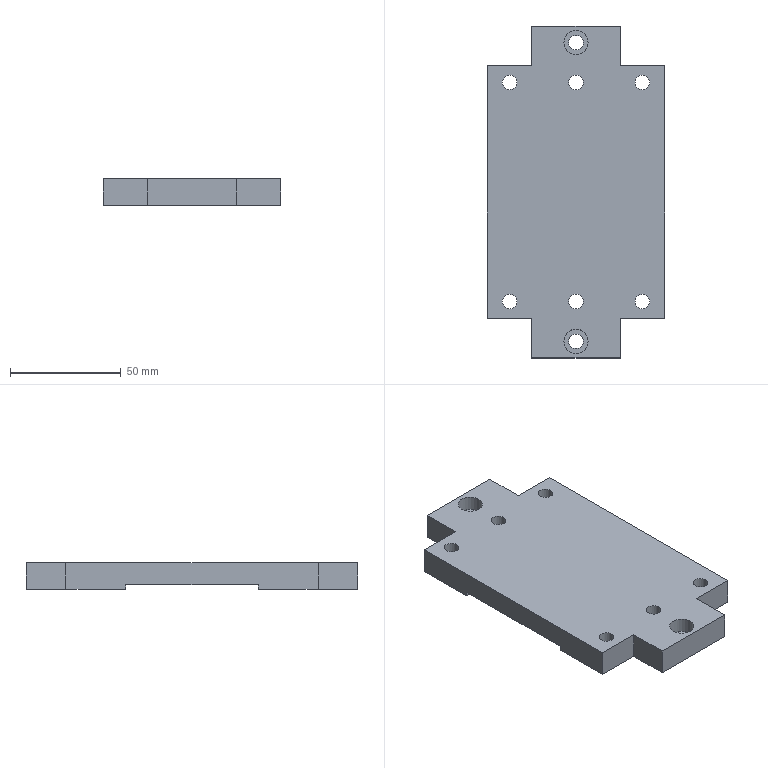Part | NX | 1 solid | 42 faces | box 80 x 150 x 12 mm | volume 110527 mm3 | plane 26 | cylinder 16 | commonest cylinder face diameters 6.6 x8 11 x8
STEP:
#1=CARTESIAN_POINT('',(5.5,67.5,6.));
#2=VERTEX_POINT('',#1);
#3=CARTESIAN_POINT('',(0.,67.5,6.));
#4=DIRECTION('',(0.,0.,1.));
#5=DIRECTION('',(1.,0.,0.));
#6=AXIS2_PLACEMENT_3D('',#3,#4,#5);
#7=CIRCLE('',#6,5.5);
#8=EDGE_CURVE('',#2,#2,#7,.T.);
#9=ORIENTED_EDGE('',*,*,#8,.F.);
#10=EDGE_LOOP('',(#9));
#11=FACE_BOUND('',#10,.T.);
#12=CARTESIAN_POINT('',(5.5,-67.5,6.));
#13=VERTEX_POINT('',#12);
#14=CARTESIAN_POINT('',(0.,-67.5,6.));
#15=DIRECTION('',(0.,0.,1.));
#16=DIRECTION('',(1.,0.,0.));
#17=AXIS2_PLACEMENT_3D('',#14,#15,#16);
#18=CIRCLE('',#17,5.5);
#19=EDGE_CURVE('',#13,#13,#18,.T.);
#20=ORIENTED_EDGE('',*,*,#19,.F.);
#21=EDGE_LOOP('',(#20));
#22=FACE_BOUND('',#21,.T.);
#23=CARTESIAN_POINT('',(-33.3,-49.5,6.));
#24=VERTEX_POINT('',#23);
#25=CARTESIAN_POINT('',(-30.,-49.5,6.));
#26=DIRECTION('',(0.,0.,-1.));
#27=DIRECTION('',(-1.,0.,0.));
#28=AXIS2_PLACEMENT_3D('',#25,#26,#27);
#29=CIRCLE('',#28,3.3);
#30=EDGE_CURVE('',#24,#24,#29,.T.);
#31=ORIENTED_EDGE('',*,*,#30,.T.);
#32=EDGE_LOOP('',(#31));
#33=FACE_BOUND('',#32,.T.);
#34=CARTESIAN_POINT('',(-3.3,-49.5,6.));
#35=VERTEX_POINT('',#34);
#36=CARTESIAN_POINT('',(0.,-49.5,6.));
#37=DIRECTION('',(0.,0.,-1.));
#38=DIRECTION('',(-1.,0.,0.));
#39=AXIS2_PLACEMENT_3D('',#36,#37,#38);
#40=CIRCLE('',#39,3.3);
#41=EDGE_CURVE('',#35,#35,#40,.T.);
#42=ORIENTED_EDGE('',*,*,#41,.T.);
#43=EDGE_LOOP('',(#42));
#44=FACE_BOUND('',#43,.T.);
#45=CARTESIAN_POINT('',(26.7,-49.5,6.));
#46=VERTEX_POINT('',#45);
#47=CARTESIAN_POINT('',(30.,-49.5,6.));
#48=DIRECTION('',(0.,0.,-1.));
#49=DIRECTION('',(-1.,0.,0.));
#50=AXIS2_PLACEMENT_3D('',#47,#48,#49);
#51=CIRCLE('',#50,3.3);
#52=EDGE_CURVE('',#46,#46,#51,.T.);
#53=ORIENTED_EDGE('',*,*,#52,.T.);
#54=EDGE_LOOP('',(#53));
#55=FACE_BOUND('',#54,.T.);
#56=CARTESIAN_POINT('',(-33.3,49.5,6.));
#57=VERTEX_POINT('',#56);
#58=CARTESIAN_POINT('',(-30.,49.5,6.));
#59=DIRECTION('',(0.,0.,-1.));
#60=DIRECTION('',(-1.,0.,0.));
#61=AXIS2_PLACEMENT_3D('',#58,#59,#60);
#62=CIRCLE('',#61,3.3);
#63=EDGE_CURVE('',#57,#57,#62,.T.);
#64=ORIENTED_EDGE('',*,*,#63,.T.);
#65=EDGE_LOOP('',(#64));
#66=FACE_BOUND('',#65,.T.);
#67=CARTESIAN_POINT('',(-3.3,49.5,6.));
#68=VERTEX_POINT('',#67);
#69=CARTESIAN_POINT('',(0.,49.5,6.));
#70=DIRECTION('',(0.,0.,-1.));
#71=DIRECTION('',(-1.,0.,0.));
#72=AXIS2_PLACEMENT_3D('',#69,#70,#71);
#73=CIRCLE('',#72,3.3);
#74=EDGE_CURVE('',#68,#68,#73,.T.);
#75=ORIENTED_EDGE('',*,*,#74,.T.);
#76=EDGE_LOOP('',(#75));
#77=FACE_BOUND('',#76,.T.);
#78=CARTESIAN_POINT('',(26.7,49.5,6.));
#79=VERTEX_POINT('',#78);
#80=CARTESIAN_POINT('',(30.,49.5,6.));
#81=DIRECTION('',(0.,0.,-1.));
#82=DIRECTION('',(-1.,0.,0.));
#83=AXIS2_PLACEMENT_3D('',#80,#81,#82);
#84=CIRCLE('',#83,3.3);
#85=EDGE_CURVE('',#79,#79,#84,.T.);
#86=ORIENTED_EDGE('',*,*,#85,.T.);
#87=EDGE_LOOP('',(#86));
#88=FACE_BOUND('',#87,.T.);
#89=CARTESIAN_POINT('',(-40.,57.,6.));
#90=VERTEX_POINT('',#89);
#91=CARTESIAN_POINT('',(-40.,-57.,6.));
#92=VERTEX_POINT('',#91);
#93=CARTESIAN_POINT('',(-40.,75.,6.));
#94=DIRECTION('',(0.,-1.,0.));
#95=VECTOR('',#94,1000.);
#96=LINE('',#93,#95);
#97=EDGE_CURVE('',#90,#92,#96,.T.);
#98=ORIENTED_EDGE('',*,*,#97,.T.);
#99=CARTESIAN_POINT('',(-20.,-57.,6.));
#100=VERTEX_POINT('',#99);
#101=CARTESIAN_POINT('',(-40.,-57.,6.));
#102=DIRECTION('',(1.,0.,0.));
#103=VECTOR('',#102,1000.);
#104=LINE('',#101,#103);
#105=EDGE_CURVE('',#92,#100,#104,.T.);
#106=ORIENTED_EDGE('',*,*,#105,.T.);
#107=CARTESIAN_POINT('',(-20.,-75.,6.));
#108=VERTEX_POINT('',#107);
#109=CARTESIAN_POINT('',(-20.,-75.,6.));
#110=DIRECTION('',(0.,-1.,0.));
#111=VECTOR('',#110,1000.);
#112=LINE('',#109,#111);
#113=EDGE_CURVE('',#100,#108,#112,.T.);
#114=ORIENTED_EDGE('',*,*,#113,.T.);
#115=CARTESIAN_POINT('',(20.,-75.,6.));
#116=VERTEX_POINT('',#115);
#117=CARTESIAN_POINT('',(-40.,-75.,6.));
#118=DIRECTION('',(1.,0.,0.));
#119=VECTOR('',#118,1000.);
#120=LINE('',#117,#119);
#121=EDGE_CURVE('',#108,#116,#120,.T.);
#122=ORIENTED_EDGE('',*,*,#121,.T.);
#123=CARTESIAN_POINT('',(20.,-57.,6.));
#124=VERTEX_POINT('',#123);
#125=CARTESIAN_POINT('',(20.,-75.,6.));
#126=DIRECTION('',(0.,-1.,0.));
#127=VECTOR('',#126,1000.);
#128=LINE('',#125,#127);
#129=EDGE_CURVE('',#124,#116,#128,.T.);
#130=ORIENTED_EDGE('',*,*,#129,.F.);
#131=CARTESIAN_POINT('',(40.,-57.,6.));
#132=VERTEX_POINT('',#131);
#133=CARTESIAN_POINT('',(40.,-57.,6.));
#134=DIRECTION('',(-1.,0.,0.));
#135=VECTOR('',#134,1000.);
#136=LINE('',#133,#135);
#137=EDGE_CURVE('',#132,#124,#136,.T.);
#138=ORIENTED_EDGE('',*,*,#137,.F.);
#139=CARTESIAN_POINT('',(40.,57.,6.));
#140=VERTEX_POINT('',#139);
#141=CARTESIAN_POINT('',(40.,75.,6.));
#142=DIRECTION('',(0.,1.,0.));
#143=VECTOR('',#142,1000.);
#144=LINE('',#141,#143);
#145=EDGE_CURVE('',#132,#140,#144,.T.);
#146=ORIENTED_EDGE('',*,*,#145,.T.);
#147=CARTESIAN_POINT('',(20.,57.,6.));
#148=VERTEX_POINT('',#147);
#149=CARTESIAN_POINT('',(40.,57.,6.));
#150=DIRECTION('',(-1.,0.,0.));
#151=VECTOR('',#150,1000.);
#152=LINE('',#149,#151);
#153=EDGE_CURVE('',#140,#148,#152,.T.);
#154=ORIENTED_EDGE('',*,*,#153,.T.);
#155=CARTESIAN_POINT('',(20.,75.,6.));
#156=VERTEX_POINT('',#155);
#157=CARTESIAN_POINT('',(20.,75.,6.));
#158=DIRECTION('',(0.,1.,0.));
#159=VECTOR('',#158,1000.);
#160=LINE('',#157,#159);
#161=EDGE_CURVE('',#148,#156,#160,.T.);
#162=ORIENTED_EDGE('',*,*,#161,.T.);
#163=CARTESIAN_POINT('',(-20.,75.,6.));
#164=VERTEX_POINT('',#163);
#165=CARTESIAN_POINT('',(-40.,75.,6.));
#166=DIRECTION('',(-1.,0.,0.));
#167=VECTOR('',#166,1000.);
#168=LINE('',#165,#167);
#169=EDGE_CURVE('',#156,#164,#168,.T.);
#170=ORIENTED_EDGE('',*,*,#169,.T.);
#171=CARTESIAN_POINT('',(-20.,57.,6.));
#172=VERTEX_POINT('',#171);
#173=CARTESIAN_POINT('',(-20.,75.,6.));
#174=DIRECTION('',(0.,1.,0.));
#175=VECTOR('',#174,1000.);
#176=LINE('',#173,#175);
#177=EDGE_CURVE('',#172,#164,#176,.T.);
#178=ORIENTED_EDGE('',*,*,#177,.F.);
#179=CARTESIAN_POINT('',(-40.,57.,6.));
#180=DIRECTION('',(1.,0.,0.));
#181=VECTOR('',#180,1000.);
#182=LINE('',#179,#181);
#183=EDGE_CURVE('',#90,#172,#182,.T.);
#184=ORIENTED_EDGE('',*,*,#183,.F.);
#185=EDGE_LOOP('',(#98,#106,#114,#122,#130,#138,#146,#154,#162,#170,#178,#184));
#186=FACE_BOUND('',#185,.T.);
#187=CARTESIAN_POINT('',(0.,0.,6.));
#188=DIRECTION('',(0.,0.,1.));
#189=DIRECTION('',(1.,0.,0.));
#190=AXIS2_PLACEMENT_3D('',#187,#188,#189);
#191=PLANE('',#190);
#192=ADVANCED_FACE('',(#11,#22,#33,#44,#55,#66,#77,#88,#186),#191,.T.);
#193=CARTESIAN_POINT('',(24.5,-49.5,-6.));
#194=VERTEX_POINT('',#193);
#195=CARTESIAN_POINT('',(30.,-49.5,-6.));
#196=DIRECTION('',(0.,0.,-1.));
#197=DIRECTION('',(-1.,0.,0.));
#198=AXIS2_PLACEMENT_3D('',#195,#196,#197);
#199=CIRCLE('',#198,5.5);
#200=EDGE_CURVE('',#194,#194,#199,.T.);
#201=ORIENTED_EDGE('',*,*,#200,.F.);
#202=EDGE_LOOP('',(#201));
#203=FACE_BOUND('',#202,.T.);
#204=CARTESIAN_POINT('',(-5.5,-49.5,-6.));
#205=VERTEX_POINT('',#204);
#206=CARTESIAN_POINT('',(0.,-49.5,-6.));
#207=DIRECTION('',(0.,0.,-1.));
#208=DIRECTION('',(-1.,0.,0.));
#209=AXIS2_PLACEMENT_3D('',#206,#207,#208);
#210=CIRCLE('',#209,5.5);
#211=EDGE_CURVE('',#205,#205,#210,.T.);
#212=ORIENTED_EDGE('',*,*,#211,.F.);
#213=EDGE_LOOP('',(#212));
#214=FACE_BOUND('',#213,.T.);
#215=CARTESIAN_POINT('',(-35.5,-49.5,-6.));
#216=VERTEX_POINT('',#215);
#217=CARTESIAN_POINT('',(-30.,-49.5,-6.));
#218=DIRECTION('',(0.,0.,-1.));
#219=DIRECTION('',(-1.,0.,0.));
#220=AXIS2_PLACEMENT_3D('',#217,#218,#219);
#221=CIRCLE('',#220,5.5);
#222=EDGE_CURVE('',#216,#216,#221,.T.);
#223=ORIENTED_EDGE('',*,*,#222,.F.);
#224=EDGE_LOOP('',(#223));
#225=FACE_BOUND('',#224,.T.);
#226=CARTESIAN_POINT('',(3.3,-67.5,-6.));
#227=VERTEX_POINT('',#226);
#228=CARTESIAN_POINT('',(0.,-67.5,-6.));
#229=DIRECTION('',(0.,0.,1.));
#230=DIRECTION('',(1.,0.,0.));
#231=AXIS2_PLACEMENT_3D('',#228,#229,#230);
#232=CIRCLE('',#231,3.3);
#233=EDGE_CURVE('',#227,#227,#232,.T.);
#234=ORIENTED_EDGE('',*,*,#233,.T.);
#235=EDGE_LOOP('',(#234));
#236=FACE_BOUND('',#235,.T.);
#237=CARTESIAN_POINT('',(-40.,-57.,-6.));
#238=VERTEX_POINT('',#237);
#239=CARTESIAN_POINT('',(-20.,-57.,-6.));
#240=VERTEX_POINT('',#239);
#241=CARTESIAN_POINT('',(-40.,-57.,-6.));
#242=DIRECTION('',(1.,0.,0.));
#243=VECTOR('',#242,1000.);
#244=LINE('',#241,#243);
#245=EDGE_CURVE('',#238,#240,#244,.T.);
#246=ORIENTED_EDGE('',*,*,#245,.F.);
#247=CARTESIAN_POINT('',(-40.,-30.,-6.));
#248=VERTEX_POINT('',#247);
#249=CARTESIAN_POINT('',(-40.,75.,-6.));
#250=DIRECTION('',(0.,-1.,0.));
#251=VECTOR('',#250,1000.);
#252=LINE('',#249,#251);
#253=EDGE_CURVE('',#248,#238,#252,.T.);
#254=ORIENTED_EDGE('',*,*,#253,.F.);
#255=CARTESIAN_POINT('',(40.,-30.,-6.));
#256=VERTEX_POINT('',#255);
#257=CARTESIAN_POINT('',(-40.,-30.,-6.));
#258=DIRECTION('',(-1.,0.,0.));
#259=VECTOR('',#258,1000.);
#260=LINE('',#257,#259);
#261=EDGE_CURVE('',#256,#248,#260,.T.);
#262=ORIENTED_EDGE('',*,*,#261,.F.);
#263=CARTESIAN_POINT('',(40.,-57.,-6.));
#264=VERTEX_POINT('',#263);
#265=CARTESIAN_POINT('',(40.,75.,-6.));
#266=DIRECTION('',(0.,1.,0.));
#267=VECTOR('',#266,1000.);
#268=LINE('',#265,#267);
#269=EDGE_CURVE('',#264,#256,#268,.T.);
#270=ORIENTED_EDGE('',*,*,#269,.F.);
#271=CARTESIAN_POINT('',(20.,-57.,-6.));
#272=VERTEX_POINT('',#271);
#273=CARTESIAN_POINT('',(40.,-57.,-6.));
#274=DIRECTION('',(-1.,0.,0.));
#275=VECTOR('',#274,1000.);
#276=LINE('',#273,#275);
#277=EDGE_CURVE('',#264,#272,#276,.T.);
#278=ORIENTED_EDGE('',*,*,#277,.T.);
#279=CARTESIAN_POINT('',(20.,-75.,-6.));
#280=VERTEX_POINT('',#279);
#281=CARTESIAN_POINT('',(20.,-75.,-6.));
#282=DIRECTION('',(0.,-1.,0.));
#283=VECTOR('',#282,1000.);
#284=LINE('',#281,#283);
#285=EDGE_CURVE('',#272,#280,#284,.T.);
#286=ORIENTED_EDGE('',*,*,#285,.T.);
#287=CARTESIAN_POINT('',(-20.,-75.,-6.));
#288=VERTEX_POINT('',#287);
#289=CARTESIAN_POINT('',(-40.,-75.,-6.));
#290=DIRECTION('',(1.,0.,0.));
#291=VECTOR('',#290,1000.);
#292=LINE('',#289,#291);
#293=EDGE_CURVE('',#288,#280,#292,.T.);
#294=ORIENTED_EDGE('',*,*,#293,.F.);
#295=CARTESIAN_POINT('',(-20.,-75.,-6.));
#296=DIRECTION('',(0.,-1.,0.));
#297=VECTOR('',#296,1000.);
#298=LINE('',#295,#297);
#299=EDGE_CURVE('',#240,#288,#298,.T.);
#300=ORIENTED_EDGE('',*,*,#299,.F.);
#301=EDGE_LOOP('',(#246,#254,#262,#270,#278,#286,#294,#300));
#302=FACE_BOUND('',#301,.T.);
#303=CARTESIAN_POINT('',(0.,0.,-6.));
#304=DIRECTION('',(0.,0.,1.));
#305=DIRECTION('',(1.,0.,0.));
#306=AXIS2_PLACEMENT_3D('',#303,#304,#305);
#307=PLANE('',#306);
#308=ADVANCED_FACE('',(#203,#214,#225,#236,#302),#307,.F.);
#309=CARTESIAN_POINT('',(-40.,-57.,-6.));
#310=DIRECTION('',(0.,0.,1.));
#311=VECTOR('',#310,1000.);
#312=LINE('',#309,#311);
#313=EDGE_CURVE('',#238,#92,#312,.T.);
#314=ORIENTED_EDGE('',*,*,#313,.T.);
#315=ORIENTED_EDGE('',*,*,#97,.F.);
#316=CARTESIAN_POINT('',(-40.,57.,-6.));
#317=VERTEX_POINT('',#316);
#318=CARTESIAN_POINT('',(-40.,57.,-6.));
#319=DIRECTION('',(0.,0.,1.));
#320=VECTOR('',#319,1000.);
#321=LINE('',#318,#320);
#322=EDGE_CURVE('',#317,#90,#321,.T.);
#323=ORIENTED_EDGE('',*,*,#322,.F.);
#324=CARTESIAN_POINT('',(-40.,30.,-6.));
#325=VERTEX_POINT('',#324);
#326=CARTESIAN_POINT('',(-40.,75.,-6.));
#327=DIRECTION('',(0.,-1.,0.));
#328=VECTOR('',#327,1000.);
#329=LINE('',#326,#328);
#330=EDGE_CURVE('',#317,#325,#329,.T.);
#331=ORIENTED_EDGE('',*,*,#330,.T.);
#332=CARTESIAN_POINT('',(-40.,30.,-4.));
#333=VERTEX_POINT('',#332);
#334=CARTESIAN_POINT('',(-40.,30.,-4.));
#335=DIRECTION('',(0.,0.,-1.));
#336=VECTOR('',#335,1000.);
#337=LINE('',#334,#336);
#338=EDGE_CURVE('',#333,#325,#337,.T.);
#339=ORIENTED_EDGE('',*,*,#338,.F.);
#340=CARTESIAN_POINT('',(-40.,-30.,-4.));
#341=VERTEX_POINT('',#340);
#342=CARTESIAN_POINT('',(-40.,30.,-4.));
#343=DIRECTION('',(0.,1.,0.));
#344=VECTOR('',#343,1000.);
#345=LINE('',#342,#344);
#346=EDGE_CURVE('',#341,#333,#345,.T.);
#347=ORIENTED_EDGE('',*,*,#346,.F.);
#348=CARTESIAN_POINT('',(-40.,-30.,-4.));
#349=DIRECTION('',(0.,0.,-1.));
#350=VECTOR('',#349,1000.);
#351=LINE('',#348,#350);
#352=EDGE_CURVE('',#341,#248,#351,.T.);
#353=ORIENTED_EDGE('',*,*,#352,.T.);
#354=ORIENTED_EDGE('',*,*,#253,.T.);
#355=EDGE_LOOP('',(#314,#315,#323,#331,#339,#347,#353,#354));
#356=FACE_BOUND('',#355,.T.);
#357=CARTESIAN_POINT('',(-40.,75.,6.));
#358=DIRECTION('',(1.,0.,0.));
#359=DIRECTION('',(0.,1.,0.));
#360=AXIS2_PLACEMENT_3D('',#357,#358,#359);
#361=PLANE('',#360);
#362=ADVANCED_FACE('',(#356),#361,.F.);
#363=CARTESIAN_POINT('',(-20.,-75.,-6.));
#364=DIRECTION('',(0.,0.,1.));
#365=VECTOR('',#364,1000.);
#366=LINE('',#363,#365);
#367=EDGE_CURVE('',#288,#108,#366,.T.);
#368=ORIENTED_EDGE('',*,*,#367,.F.);
#369=ORIENTED_EDGE('',*,*,#293,.T.);
#370=CARTESIAN_POINT('',(20.,-75.,-6.));
#371=DIRECTION('',(0.,0.,1.));
#372=VECTOR('',#371,1000.);
#373=LINE('',#370,#372);
#374=EDGE_CURVE('',#280,#116,#373,.T.);
#375=ORIENTED_EDGE('',*,*,#374,.T.);
#376=ORIENTED_EDGE('',*,*,#121,.F.);
#377=EDGE_LOOP('',(#368,#369,#375,#376));
#378=FACE_BOUND('',#377,.T.);
#379=CARTESIAN_POINT('',(-40.,-75.,6.));
#380=DIRECTION('',(0.,1.,0.));
#381=DIRECTION('',(0.,0.,1.));
#382=AXIS2_PLACEMENT_3D('',#379,#380,#381);
#383=PLANE('',#382);
#384=ADVANCED_FACE('',(#378),#383,.F.);
#385=CARTESIAN_POINT('',(40.,57.,-6.));
#386=VERTEX_POINT('',#385);
#387=CARTESIAN_POINT('',(40.,57.,-6.));
#388=DIRECTION('',(0.,0.,1.));
#389=VECTOR('',#388,1000.);
#390=LINE('',#387,#389);
#391=EDGE_CURVE('',#386,#140,#390,.T.);
#392=ORIENTED_EDGE('',*,*,#391,.T.);
#393=ORIENTED_EDGE('',*,*,#145,.F.);
#394=CARTESIAN_POINT('',(40.,-57.,-6.));
#395=DIRECTION('',(0.,0.,1.));
#396=VECTOR('',#395,1000.);
#397=LINE('',#394,#396);
#398=EDGE_CURVE('',#264,#132,#397,.T.);
#399=ORIENTED_EDGE('',*,*,#398,.F.);
#400=ORIENTED_EDGE('',*,*,#269,.T.);
#401=CARTESIAN_POINT('',(40.,-30.,-4.));
#402=VERTEX_POINT('',#401);
#403=CARTESIAN_POINT('',(40.,-30.,-4.));
#404=DIRECTION('',(0.,0.,-1.));
#405=VECTOR('',#404,1000.);
#406=LINE('',#403,#405);
#407=EDGE_CURVE('',#402,#256,#406,.T.);
#408=ORIENTED_EDGE('',*,*,#407,.F.);
#409=CARTESIAN_POINT('',(40.,30.,-4.));
#410=VERTEX_POINT('',#409);
#411=CARTESIAN_POINT('',(40.,30.,-4.));
#412=DIRECTION('',(0.,-1.,0.));
#413=VECTOR('',#412,1000.);
#414=LINE('',#411,#413);
#415=EDGE_CURVE('',#410,#402,#414,.T.);
#416=ORIENTED_EDGE('',*,*,#415,.F.);
#417=CARTESIAN_POINT('',(40.,30.,-6.));
#418=VERTEX_POINT('',#417);
#419=CARTESIAN_POINT('',(40.,30.,-4.));
#420=DIRECTION('',(0.,0.,-1.));
#421=VECTOR('',#420,1000.);
#422=LINE('',#419,#421);
#423=EDGE_CURVE('',#410,#418,#422,.T.);
#424=ORIENTED_EDGE('',*,*,#423,.T.);
#425=CARTESIAN_POINT('',(40.,75.,-6.));
#426=DIRECTION('',(0.,1.,0.));
#427=VECTOR('',#426,1000.);
#428=LINE('',#425,#427);
#429=EDGE_CURVE('',#418,#386,#428,.T.);
#430=ORIENTED_EDGE('',*,*,#429,.T.);
#431=EDGE_LOOP('',(#392,#393,#399,#400,#408,#416,#424,#430));
#432=FACE_BOUND('',#431,.T.);
#433=CARTESIAN_POINT('',(40.,75.,6.));
#434=DIRECTION('',(-1.,0.,0.));
#435=DIRECTION('',(0.,-1.,0.));
#436=AXIS2_PLACEMENT_3D('',#433,#434,#435);
#437=PLANE('',#436);
#438=ADVANCED_FACE('',(#432),#437,.F.);
#439=CARTESIAN_POINT('',(20.,75.,-6.));
#440=VERTEX_POINT('',#439);
#441=CARTESIAN_POINT('',(-20.,75.,-6.));
#442=VERTEX_POINT('',#441);
#443=CARTESIAN_POINT('',(-40.,75.,-6.));
#444=DIRECTION('',(-1.,0.,0.));
#445=VECTOR('',#444,1000.);
#446=LINE('',#443,#445);
#447=EDGE_CURVE('',#440,#442,#446,.T.);
#448=ORIENTED_EDGE('',*,*,#447,.T.);
#449=CARTESIAN_POINT('',(-20.,75.,-6.));
#450=DIRECTION('',(0.,0.,1.));
#451=VECTOR('',#450,1000.);
#452=LINE('',#449,#451);
#453=EDGE_CURVE('',#442,#164,#452,.T.);
#454=ORIENTED_EDGE('',*,*,#453,.T.);
#455=ORIENTED_EDGE('',*,*,#169,.F.);
#456=CARTESIAN_POINT('',(20.,75.,-6.));
#457=DIRECTION('',(0.,0.,1.));
#458=VECTOR('',#457,1000.);
#459=LINE('',#456,#458);
#460=EDGE_CURVE('',#440,#156,#459,.T.);
#461=ORIENTED_EDGE('',*,*,#460,.F.);
#462=EDGE_LOOP('',(#448,#454,#455,#461));
#463=FACE_BOUND('',#462,.T.);
#464=CARTESIAN_POINT('',(-40.,75.,6.));
#465=DIRECTION('',(0.,-1.,0.));
#466=DIRECTION('',(0.,0.,-1.));
#467=AXIS2_PLACEMENT_3D('',#464,#465,#466);
#468=PLANE('',#467);
#469=ADVANCED_FACE('',(#463),#468,.F.);
#470=CARTESIAN_POINT('',(24.5,49.5,-6.));
#471=VERTEX_POINT('',#470);
#472=CARTESIAN_POINT('',(30.,49.5,-6.));
#473=DIRECTION('',(0.,0.,-1.));
#474=DIRECTION('',(-1.,0.,0.));
#475=AXIS2_PLACEMENT_3D('',#472,#473,#474);
#476=CIRCLE('',#475,5.5);
#477=EDGE_CURVE('',#471,#471,#476,.T.);
#478=ORIENTED_EDGE('',*,*,#477,.F.);
#479=EDGE_LOOP('',(#478));
#480=FACE_BOUND('',#479,.T.);
#481=CARTESIAN_POINT('',(-5.5,49.5,-6.));
#482=VERTEX_POINT('',#481);
#483=CARTESIAN_POINT('',(0.,49.5,-6.));
#484=DIRECTION('',(0.,0.,-1.));
#485=DIRECTION('',(-1.,0.,0.));
#486=AXIS2_PLACEMENT_3D('',#483,#484,#485);
#487=CIRCLE('',#486,5.5);
#488=EDGE_CURVE('',#482,#482,#487,.T.);
#489=ORIENTED_EDGE('',*,*,#488,.F.);
#490=EDGE_LOOP('',(#489));
#491=FACE_BOUND('',#490,.T.);
#492=CARTESIAN_POINT('',(-35.5,49.5,-6.));
#493=VERTEX_POINT('',#492);
#494=CARTESIAN_POINT('',(-30.,49.5,-6.));
#495=DIRECTION('',(0.,0.,-1.));
#496=DIRECTION('',(-1.,0.,0.));
#497=AXIS2_PLACEMENT_3D('',#494,#495,#496);
#498=CIRCLE('',#497,5.5);
#499=EDGE_CURVE('',#493,#493,#498,.T.);
#500=ORIENTED_EDGE('',*,*,#499,.F.);
#501=EDGE_LOOP('',(#500));
#502=FACE_BOUND('',#501,.T.);
#503=CARTESIAN_POINT('',(3.3,67.5,-6.));
#504=VERTEX_POINT('',#503);
#505=CARTESIAN_POINT('',(0.,67.5,-6.));
#506=DIRECTION('',(0.,0.,1.));
#507=DIRECTION('',(1.,0.,0.));
#508=AXIS2_PLACEMENT_3D('',#505,#506,#507);
#509=CIRCLE('',#508,3.3);
#510=EDGE_CURVE('',#504,#504,#509,.T.);
#511=ORIENTED_EDGE('',*,*,#510,.T.);
#512=EDGE_LOOP('',(#511));
#513=FACE_BOUND('',#512,.T.);
#514=CARTESIAN_POINT('',(-20.,57.,-6.));
#515=VERTEX_POINT('',#514);
#516=CARTESIAN_POINT('',(-40.,57.,-6.));
#517=DIRECTION('',(1.,0.,0.));
#518=VECTOR('',#517,1000.);
#519=LINE('',#516,#518);
#520=EDGE_CURVE('',#317,#515,#519,.T.);
#521=ORIENTED_EDGE('',*,*,#520,.T.);
#522=CARTESIAN_POINT('',(-20.,75.,-6.));
#523=DIRECTION('',(0.,1.,0.));
#524=VECTOR('',#523,1000.);
#525=LINE('',#522,#524);
#526=EDGE_CURVE('',#515,#442,#525,.T.);
#527=ORIENTED_EDGE('',*,*,#526,.T.);
#528=ORIENTED_EDGE('',*,*,#447,.F.);
#529=CARTESIAN_POINT('',(20.,57.,-6.));
#530=VERTEX_POINT('',#529);
#531=CARTESIAN_POINT('',(20.,75.,-6.));
#532=DIRECTION('',(0.,1.,0.));
#533=VECTOR('',#532,1000.);
#534=LINE('',#531,#533);
#535=EDGE_CURVE('',#530,#440,#534,.T.);
#536=ORIENTED_EDGE('',*,*,#535,.F.);
#537=CARTESIAN_POINT('',(40.,57.,-6.));
#538=DIRECTION('',(-1.,0.,0.));
#539=VECTOR('',#538,1000.);
#540=LINE('',#537,#539);
#541=EDGE_CURVE('',#386,#530,#540,.T.);
#542=ORIENTED_EDGE('',*,*,#541,.F.);
#543=ORIENTED_EDGE('',*,*,#429,.F.);
#544=CARTESIAN_POINT('',(-40.,30.,-6.));
#545=DIRECTION('',(1.,0.,0.));
#546=VECTOR('',#545,1000.);
#547=LINE('',#544,#546);
#548=EDGE_CURVE('',#325,#418,#547,.T.);
#549=ORIENTED_EDGE('',*,*,#548,.F.);
#550=ORIENTED_EDGE('',*,*,#330,.F.);
#551=EDGE_LOOP('',(#521,#527,#528,#536,#542,#543,#549,#550));
#552=FACE_BOUND('',#551,.T.);
#553=CARTESIAN_POINT('',(0.,0.,-6.));
#554=DIRECTION('',(0.,0.,1.));
#555=DIRECTION('',(1.,0.,0.));
#556=AXIS2_PLACEMENT_3D('',#553,#554,#555);
#557=PLANE('',#556);
#558=ADVANCED_FACE('',(#480,#491,#502,#513,#552),#557,.F.);
#559=ORIENTED_EDGE('',*,*,#261,.T.);
#560=ORIENTED_EDGE('',*,*,#352,.F.);
#561=CARTESIAN_POINT('',(-40.,-30.,-4.));
#562=DIRECTION('',(-1.,0.,0.));
#563=VECTOR('',#562,1000.);
#564=LINE('',#561,#563);
#565=EDGE_CURVE('',#402,#341,#564,.T.);
#566=ORIENTED_EDGE('',*,*,#565,.F.);
#567=ORIENTED_EDGE('',*,*,#407,.T.);
#568=EDGE_LOOP('',(#559,#560,#566,#567));
#569=FACE_BOUND('',#568,.T.);
#570=CARTESIAN_POINT('',(-40.,-30.,-4.));
#571=DIRECTION('',(0.,-1.,0.));
#572=DIRECTION('',(1.,0.,0.));
#573=AXIS2_PLACEMENT_3D('',#570,#571,#572);
#574=PLANE('',#573);
#575=ADVANCED_FACE('',(#569),#574,.F.);
#576=ORIENTED_EDGE('',*,*,#548,.T.);
#577=ORIENTED_EDGE('',*,*,#423,.F.);
#578=CARTESIAN_POINT('',(-40.,30.,-4.));
#579=DIRECTION('',(1.,0.,0.));
#580=VECTOR('',#579,1000.);
#581=LINE('',#578,#580);
#582=EDGE_CURVE('',#333,#410,#581,.T.);
#583=ORIENTED_EDGE('',*,*,#582,.F.);
#584=ORIENTED_EDGE('',*,*,#338,.T.);
#585=EDGE_LOOP('',(#576,#577,#583,#584));
#586=FACE_BOUND('',#585,.T.);
#587=CARTESIAN_POINT('',(-40.,30.,-4.));
#588=DIRECTION('',(0.,1.,0.));
#589=DIRECTION('',(-1.,0.,0.));
#590=AXIS2_PLACEMENT_3D('',#587,#588,#589);
#591=PLANE('',#590);
#592=ADVANCED_FACE('',(#586),#591,.F.);
#593=ORIENTED_EDGE('',*,*,#346,.T.);
#594=ORIENTED_EDGE('',*,*,#582,.T.);
#595=ORIENTED_EDGE('',*,*,#415,.T.);
#596=ORIENTED_EDGE('',*,*,#565,.T.);
#597=EDGE_LOOP('',(#593,#594,#595,#596));
#598=FACE_BOUND('',#597,.T.);
#599=CARTESIAN_POINT('',(0.,0.,-4.));
#600=DIRECTION('',(0.,0.,1.));
#601=DIRECTION('',(1.,0.,0.));
#602=AXIS2_PLACEMENT_3D('',#599,#600,#601);
#603=PLANE('',#602);
#604=ADVANCED_FACE('',(#598),#603,.F.);
#605=ORIENTED_EDGE('',*,*,#85,.F.);
#606=EDGE_LOOP('',(#605));
#607=FACE_BOUND('',#606,.T.);
#608=CARTESIAN_POINT('',(26.7,49.5,0.8));
#609=VERTEX_POINT('',#608);
#610=CARTESIAN_POINT('',(30.,49.5,0.8));
#611=DIRECTION('',(0.,0.,-1.));
#612=DIRECTION('',(-1.,0.,0.));
#613=AXIS2_PLACEMENT_3D('',#610,#611,#612);
#614=CIRCLE('',#613,3.3);
#615=EDGE_CURVE('',#609,#609,#614,.T.);
#616=ORIENTED_EDGE('',*,*,#615,.T.);
#617=EDGE_LOOP('',(#616));
#618=FACE_BOUND('',#617,.T.);
#619=CARTESIAN_POINT('',(30.,49.5,-6.));
#620=DIRECTION('',(0.,0.,-1.));
#621=DIRECTION('',(-1.,0.,0.));
#622=AXIS2_PLACEMENT_3D('',#619,#620,#621);
#623=CYLINDRICAL_SURFACE('',#622,3.3);
#624=ADVANCED_FACE('',(#607,#618),#623,.F.);
#625=ORIENTED_EDGE('',*,*,#615,.F.);
#626=EDGE_LOOP('',(#625));
#627=FACE_BOUND('',#626,.T.);
#628=CARTESIAN_POINT('',(24.5,49.5,0.8));
#629=VERTEX_POINT('',#628);
#630=CARTESIAN_POINT('',(30.,49.5,0.8));
#631=DIRECTION('',(0.,0.,-1.));
#632=DIRECTION('',(-1.,0.,0.));
#633=AXIS2_PLACEMENT_3D('',#630,#631,#632);
#634=CIRCLE('',#633,5.5);
#635=EDGE_CURVE('',#629,#629,#634,.T.);
#636=ORIENTED_EDGE('',*,*,#635,.T.);
#637=EDGE_LOOP('',(#636));
#638=FACE_BOUND('',#637,.T.);
#639=CARTESIAN_POINT('',(33.3,49.5,0.8));
#640=DIRECTION('',(0.,0.,1.));
#641=DIRECTION('',(1.,0.,0.));
#642=AXIS2_PLACEMENT_3D('',#639,#640,#641);
#643=PLANE('',#642);
#644=ADVANCED_FACE('',(#627,#638),#643,.F.);
#645=ORIENTED_EDGE('',*,*,#635,.F.);
#646=EDGE_LOOP('',(#645));
#647=FACE_BOUND('',#646,.T.);
#648=ORIENTED_EDGE('',*,*,#477,.T.);
#649=EDGE_LOOP('',(#648));
#650=FACE_BOUND('',#649,.T.);
#651=CARTESIAN_POINT('',(30.,49.5,-6.));
#652=DIRECTION('',(0.,0.,-1.));
#653=DIRECTION('',(-1.,0.,0.));
#654=AXIS2_PLACEMENT_3D('',#651,#652,#653);
#655=CYLINDRICAL_SURFACE('',#654,5.5);
#656=ADVANCED_FACE('',(#647,#650),#655,.F.);
#657=ORIENTED_EDGE('',*,*,#74,.F.);
#658=EDGE_LOOP('',(#657));
#659=FACE_BOUND('',#658,.T.);
#660=CARTESIAN_POINT('',(-3.3,49.5,0.8));
#661=VERTEX_POINT('',#660);
#662=CARTESIAN_POINT('',(0.,49.5,0.8));
#663=DIRECTION('',(0.,0.,-1.));
#664=DIRECTION('',(-1.,0.,0.));
#665=AXIS2_PLACEMENT_3D('',#662,#663,#664);
#666=CIRCLE('',#665,3.3);
#667=EDGE_CURVE('',#661,#661,#666,.T.);
#668=ORIENTED_EDGE('',*,*,#667,.T.);
#669=EDGE_LOOP('',(#668));
#670=FACE_BOUND('',#669,.T.);
#671=CARTESIAN_POINT('',(0.,49.5,-6.));
#672=DIRECTION('',(0.,0.,-1.));
#673=DIRECTION('',(-1.,0.,0.));
#674=AXIS2_PLACEMENT_3D('',#671,#672,#673);
#675=CYLINDRICAL_SURFACE('',#674,3.3);
#676=ADVANCED_FACE('',(#659,#670),#675,.F.);
#677=ORIENTED_EDGE('',*,*,#667,.F.);
#678=EDGE_LOOP('',(#677));
#679=FACE_BOUND('',#678,.T.);
#680=CARTESIAN_POINT('',(-5.5,49.5,0.8));
#681=VERTEX_POINT('',#680);
#682=CARTESIAN_POINT('',(0.,49.5,0.8));
#683=DIRECTION('',(0.,0.,-1.));
#684=DIRECTION('',(-1.,0.,0.));
#685=AXIS2_PLACEMENT_3D('',#682,#683,#684);
#686=CIRCLE('',#685,5.5);
#687=EDGE_CURVE('',#681,#681,#686,.T.);
#688=ORIENTED_EDGE('',*,*,#687,.T.);
#689=EDGE_LOOP('',(#688));
#690=FACE_BOUND('',#689,.T.);
#691=CARTESIAN_POINT('',(3.3,49.5,0.8));
#692=DIRECTION('',(0.,0.,1.));
#693=DIRECTION('',(1.,0.,0.));
#694=AXIS2_PLACEMENT_3D('',#691,#692,#693);
#695=PLANE('',#694);
#696=ADVANCED_FACE('',(#679,#690),#695,.F.);
#697=ORIENTED_EDGE('',*,*,#687,.F.);
#698=EDGE_LOOP('',(#697));
#699=FACE_BOUND('',#698,.T.);
#700=ORIENTED_EDGE('',*,*,#488,.T.);
#701=EDGE_LOOP('',(#700));
#702=FACE_BOUND('',#701,.T.);
#703=CARTESIAN_POINT('',(0.,49.5,-6.));
#704=DIRECTION('',(0.,0.,-1.));
#705=DIRECTION('',(-1.,0.,0.));
#706=AXIS2_PLACEMENT_3D('',#703,#704,#705);
#707=CYLINDRICAL_SURFACE('',#706,5.5);
#708=ADVANCED_FACE('',(#699,#702),#707,.F.);
#709=ORIENTED_EDGE('',*,*,#63,.F.);
#710=EDGE_LOOP('',(#709));
#711=FACE_BOUND('',#710,.T.);
#712=CARTESIAN_POINT('',(-33.3,49.5,0.8));
#713=VERTEX_POINT('',#712);
#714=CARTESIAN_POINT('',(-30.,49.5,0.8));
#715=DIRECTION('',(0.,0.,-1.));
#716=DIRECTION('',(-1.,0.,0.));
#717=AXIS2_PLACEMENT_3D('',#714,#715,#716);
#718=CIRCLE('',#717,3.3);
#719=EDGE_CURVE('',#713,#713,#718,.T.);
#720=ORIENTED_EDGE('',*,*,#719,.T.);
#721=EDGE_LOOP('',(#720));
#722=FACE_BOUND('',#721,.T.);
#723=CARTESIAN_POINT('',(-30.,49.5,-6.));
#724=DIRECTION('',(0.,0.,-1.));
#725=DIRECTION('',(-1.,0.,0.));
#726=AXIS2_PLACEMENT_3D('',#723,#724,#725);
#727=CYLINDRICAL_SURFACE('',#726,3.3);
#728=ADVANCED_FACE('',(#711,#722),#727,.F.);
#729=ORIENTED_EDGE('',*,*,#719,.F.);
#730=EDGE_LOOP('',(#729));
#731=FACE_BOUND('',#730,.T.);
#732=CARTESIAN_POINT('',(-35.5,49.5,0.8));
#733=VERTEX_POINT('',#732);
#734=CARTESIAN_POINT('',(-30.,49.5,0.8));
#735=DIRECTION('',(0.,0.,-1.));
#736=DIRECTION('',(-1.,0.,0.));
#737=AXIS2_PLACEMENT_3D('',#734,#735,#736);
#738=CIRCLE('',#737,5.5);
#739=EDGE_CURVE('',#733,#733,#738,.T.);
#740=ORIENTED_EDGE('',*,*,#739,.T.);
#741=EDGE_LOOP('',(#740));
#742=FACE_BOUND('',#741,.T.);
#743=CARTESIAN_POINT('',(-26.7,49.5,0.8));
#744=DIRECTION('',(0.,0.,1.));
#745=DIRECTION('',(1.,0.,0.));
#746=AXIS2_PLACEMENT_3D('',#743,#744,#745);
#747=PLANE('',#746);
#748=ADVANCED_FACE('',(#731,#742),#747,.F.);
#749=ORIENTED_EDGE('',*,*,#739,.F.);
#750=EDGE_LOOP('',(#749));
#751=FACE_BOUND('',#750,.T.);
#752=ORIENTED_EDGE('',*,*,#499,.T.);
#753=EDGE_LOOP('',(#752));
#754=FACE_BOUND('',#753,.T.);
#755=CARTESIAN_POINT('',(-30.,49.5,-6.));
#756=DIRECTION('',(0.,0.,-1.));
#757=DIRECTION('',(-1.,0.,0.));
#758=AXIS2_PLACEMENT_3D('',#755,#756,#757);
#759=CYLINDRICAL_SURFACE('',#758,5.5);
#760=ADVANCED_FACE('',(#751,#754),#759,.F.);
#761=ORIENTED_EDGE('',*,*,#52,.F.);
#762=EDGE_LOOP('',(#761));
#763=FACE_BOUND('',#762,.T.);
#764=CARTESIAN_POINT('',(26.7,-49.5,0.8));
#765=VERTEX_POINT('',#764);
#766=CARTESIAN_POINT('',(30.,-49.5,0.8));
#767=DIRECTION('',(0.,0.,-1.));
#768=DIRECTION('',(-1.,0.,0.));
#769=AXIS2_PLACEMENT_3D('',#766,#767,#768);
#770=CIRCLE('',#769,3.3);
#771=EDGE_CURVE('',#765,#765,#770,.T.);
#772=ORIENTED_EDGE('',*,*,#771,.T.);
#773=EDGE_LOOP('',(#772));
#774=FACE_BOUND('',#773,.T.);
#775=CARTESIAN_POINT('',(30.,-49.5,-6.));
#776=DIRECTION('',(0.,0.,-1.));
#777=DIRECTION('',(-1.,0.,0.));
#778=AXIS2_PLACEMENT_3D('',#775,#776,#777);
#779=CYLINDRICAL_SURFACE('',#778,3.3);
#780=ADVANCED_FACE('',(#763,#774),#779,.F.);
#781=ORIENTED_EDGE('',*,*,#771,.F.);
#782=EDGE_LOOP('',(#781));
#783=FACE_BOUND('',#782,.T.);
#784=CARTESIAN_POINT('',(24.5,-49.5,0.8));
#785=VERTEX_POINT('',#784);
#786=CARTESIAN_POINT('',(30.,-49.5,0.8));
#787=DIRECTION('',(0.,0.,-1.));
#788=DIRECTION('',(-1.,0.,0.));
#789=AXIS2_PLACEMENT_3D('',#786,#787,#788);
#790=CIRCLE('',#789,5.5);
#791=EDGE_CURVE('',#785,#785,#790,.T.);
#792=ORIENTED_EDGE('',*,*,#791,.T.);
#793=EDGE_LOOP('',(#792));
#794=FACE_BOUND('',#793,.T.);
#795=CARTESIAN_POINT('',(33.3,-49.5,0.8));
#796=DIRECTION('',(0.,0.,1.));
#797=DIRECTION('',(1.,0.,0.));
#798=AXIS2_PLACEMENT_3D('',#795,#796,#797);
#799=PLANE('',#798);
#800=ADVANCED_FACE('',(#783,#794),#799,.F.);
#801=ORIENTED_EDGE('',*,*,#791,.F.);
#802=EDGE_LOOP('',(#801));
#803=FACE_BOUND('',#802,.T.);
#804=ORIENTED_EDGE('',*,*,#200,.T.);
#805=EDGE_LOOP('',(#804));
#806=FACE_BOUND('',#805,.T.);
#807=CARTESIAN_POINT('',(30.,-49.5,-6.));
#808=DIRECTION('',(0.,0.,-1.));
#809=DIRECTION('',(-1.,0.,0.));
#810=AXIS2_PLACEMENT_3D('',#807,#808,#809);
#811=CYLINDRICAL_SURFACE('',#810,5.5);
#812=ADVANCED_FACE('',(#803,#806),#811,.F.);
#813=ORIENTED_EDGE('',*,*,#41,.F.);
#814=EDGE_LOOP('',(#813));
#815=FACE_BOUND('',#814,.T.);
#816=CARTESIAN_POINT('',(-3.3,-49.5,0.8));
#817=VERTEX_POINT('',#816);
#818=CARTESIAN_POINT('',(0.,-49.5,0.8));
#819=DIRECTION('',(0.,0.,-1.));
#820=DIRECTION('',(-1.,0.,0.));
#821=AXIS2_PLACEMENT_3D('',#818,#819,#820);
#822=CIRCLE('',#821,3.3);
#823=EDGE_CURVE('',#817,#817,#822,.T.);
#824=ORIENTED_EDGE('',*,*,#823,.T.);
#825=EDGE_LOOP('',(#824));
#826=FACE_BOUND('',#825,.T.);
#827=CARTESIAN_POINT('',(0.,-49.5,-6.));
#828=DIRECTION('',(0.,0.,-1.));
#829=DIRECTION('',(-1.,0.,0.));
#830=AXIS2_PLACEMENT_3D('',#827,#828,#829);
#831=CYLINDRICAL_SURFACE('',#830,3.3);
#832=ADVANCED_FACE('',(#815,#826),#831,.F.);
#833=ORIENTED_EDGE('',*,*,#823,.F.);
#834=EDGE_LOOP('',(#833));
#835=FACE_BOUND('',#834,.T.);
#836=CARTESIAN_POINT('',(-5.5,-49.5,0.8));
#837=VERTEX_POINT('',#836);
#838=CARTESIAN_POINT('',(0.,-49.5,0.8));
#839=DIRECTION('',(0.,0.,-1.));
#840=DIRECTION('',(-1.,0.,0.));
#841=AXIS2_PLACEMENT_3D('',#838,#839,#840);
#842=CIRCLE('',#841,5.5);
#843=EDGE_CURVE('',#837,#837,#842,.T.);
#844=ORIENTED_EDGE('',*,*,#843,.T.);
#845=EDGE_LOOP('',(#844));
#846=FACE_BOUND('',#845,.T.);
#847=CARTESIAN_POINT('',(3.3,-49.5,0.8));
#848=DIRECTION('',(0.,0.,1.));
#849=DIRECTION('',(1.,0.,0.));
#850=AXIS2_PLACEMENT_3D('',#847,#848,#849);
#851=PLANE('',#850);
#852=ADVANCED_FACE('',(#835,#846),#851,.F.);
#853=ORIENTED_EDGE('',*,*,#843,.F.);
#854=EDGE_LOOP('',(#853));
#855=FACE_BOUND('',#854,.T.);
#856=ORIENTED_EDGE('',*,*,#211,.T.);
#857=EDGE_LOOP('',(#856));
#858=FACE_BOUND('',#857,.T.);
#859=CARTESIAN_POINT('',(0.,-49.5,-6.));
#860=DIRECTION('',(0.,0.,-1.));
#861=DIRECTION('',(-1.,0.,0.));
#862=AXIS2_PLACEMENT_3D('',#859,#860,#861);
#863=CYLINDRICAL_SURFACE('',#862,5.5);
#864=ADVANCED_FACE('',(#855,#858),#863,.F.);
#865=ORIENTED_EDGE('',*,*,#30,.F.);
#866=EDGE_LOOP('',(#865));
#867=FACE_BOUND('',#866,.T.);
#868=CARTESIAN_POINT('',(-33.3,-49.5,0.8));
#869=VERTEX_POINT('',#868);
#870=CARTESIAN_POINT('',(-30.,-49.5,0.8));
#871=DIRECTION('',(0.,0.,-1.));
#872=DIRECTION('',(-1.,0.,0.));
#873=AXIS2_PLACEMENT_3D('',#870,#871,#872);
#874=CIRCLE('',#873,3.3);
#875=EDGE_CURVE('',#869,#869,#874,.T.);
#876=ORIENTED_EDGE('',*,*,#875,.T.);
#877=EDGE_LOOP('',(#876));
#878=FACE_BOUND('',#877,.T.);
#879=CARTESIAN_POINT('',(-30.,-49.5,-6.));
#880=DIRECTION('',(0.,0.,-1.));
#881=DIRECTION('',(-1.,0.,0.));
#882=AXIS2_PLACEMENT_3D('',#879,#880,#881);
#883=CYLINDRICAL_SURFACE('',#882,3.3);
#884=ADVANCED_FACE('',(#867,#878),#883,.F.);
#885=ORIENTED_EDGE('',*,*,#875,.F.);
#886=EDGE_LOOP('',(#885));
#887=FACE_BOUND('',#886,.T.);
#888=CARTESIAN_POINT('',(-35.5,-49.5,0.8));
#889=VERTEX_POINT('',#888);
#890=CARTESIAN_POINT('',(-30.,-49.5,0.8));
#891=DIRECTION('',(0.,0.,-1.));
#892=DIRECTION('',(-1.,0.,0.));
#893=AXIS2_PLACEMENT_3D('',#890,#891,#892);
#894=CIRCLE('',#893,5.5);
#895=EDGE_CURVE('',#889,#889,#894,.T.);
#896=ORIENTED_EDGE('',*,*,#895,.T.);
#897=EDGE_LOOP('',(#896));
#898=FACE_BOUND('',#897,.T.);
#899=CARTESIAN_POINT('',(-26.7,-49.5,0.8));
#900=DIRECTION('',(0.,0.,1.));
#901=DIRECTION('',(1.,0.,0.));
#902=AXIS2_PLACEMENT_3D('',#899,#900,#901);
#903=PLANE('',#902);
#904=ADVANCED_FACE('',(#887,#898),#903,.F.);
#905=ORIENTED_EDGE('',*,*,#895,.F.);
#906=EDGE_LOOP('',(#905));
#907=FACE_BOUND('',#906,.T.);
#908=ORIENTED_EDGE('',*,*,#222,.T.);
#909=EDGE_LOOP('',(#908));
#910=FACE_BOUND('',#909,.T.);
#911=CARTESIAN_POINT('',(-30.,-49.5,-6.));
#912=DIRECTION('',(0.,0.,-1.));
#913=DIRECTION('',(-1.,0.,0.));
#914=AXIS2_PLACEMENT_3D('',#911,#912,#913);
#915=CYLINDRICAL_SURFACE('',#914,5.5);
#916=ADVANCED_FACE('',(#907,#910),#915,.F.);
#917=ORIENTED_EDGE('',*,*,#233,.F.);
#918=EDGE_LOOP('',(#917));
#919=FACE_BOUND('',#918,.T.);
#920=CARTESIAN_POINT('',(3.3,-67.5,-0.8));
#921=VERTEX_POINT('',#920);
#922=CARTESIAN_POINT('',(0.,-67.5,-0.8));
#923=DIRECTION('',(0.,0.,1.));
#924=DIRECTION('',(1.,0.,0.));
#925=AXIS2_PLACEMENT_3D('',#922,#923,#924);
#926=CIRCLE('',#925,3.3);
#927=EDGE_CURVE('',#921,#921,#926,.T.);
#928=ORIENTED_EDGE('',*,*,#927,.T.);
#929=EDGE_LOOP('',(#928));
#930=FACE_BOUND('',#929,.T.);
#931=CARTESIAN_POINT('',(0.,-67.5,6.));
#932=DIRECTION('',(0.,0.,1.));
#933=DIRECTION('',(1.,0.,0.));
#934=AXIS2_PLACEMENT_3D('',#931,#932,#933);
#935=CYLINDRICAL_SURFACE('',#934,3.3);
#936=ADVANCED_FACE('',(#919,#930),#935,.F.);
#937=ORIENTED_EDGE('',*,*,#927,.F.);
#938=EDGE_LOOP('',(#937));
#939=FACE_BOUND('',#938,.T.);
#940=CARTESIAN_POINT('',(5.5,-67.5,-0.8));
#941=VERTEX_POINT('',#940);
#942=CARTESIAN_POINT('',(0.,-67.5,-0.8));
#943=DIRECTION('',(0.,0.,1.));
#944=DIRECTION('',(1.,0.,0.));
#945=AXIS2_PLACEMENT_3D('',#942,#943,#944);
#946=CIRCLE('',#945,5.5);
#947=EDGE_CURVE('',#941,#941,#946,.T.);
#948=ORIENTED_EDGE('',*,*,#947,.T.);
#949=EDGE_LOOP('',(#948));
#950=FACE_BOUND('',#949,.T.);
#951=CARTESIAN_POINT('',(3.3,-67.5,-0.8));
#952=DIRECTION('',(0.,0.,-1.));
#953=DIRECTION('',(-1.,0.,0.));
#954=AXIS2_PLACEMENT_3D('',#951,#952,#953);
#955=PLANE('',#954);
#956=ADVANCED_FACE('',(#939,#950),#955,.F.);
#957=ORIENTED_EDGE('',*,*,#947,.F.);
#958=EDGE_LOOP('',(#957));
#959=FACE_BOUND('',#958,.T.);
#960=ORIENTED_EDGE('',*,*,#19,.T.);
#961=EDGE_LOOP('',(#960));
#962=FACE_BOUND('',#961,.T.);
#963=CARTESIAN_POINT('',(0.,-67.5,6.));
#964=DIRECTION('',(0.,0.,1.));
#965=DIRECTION('',(1.,0.,0.));
#966=AXIS2_PLACEMENT_3D('',#963,#964,#965);
#967=CYLINDRICAL_SURFACE('',#966,5.5);
#968=ADVANCED_FACE('',(#959,#962),#967,.F.);
#969=ORIENTED_EDGE('',*,*,#510,.F.);
#970=EDGE_LOOP('',(#969));
#971=FACE_BOUND('',#970,.T.);
#972=CARTESIAN_POINT('',(3.3,67.5,-0.8));
#973=VERTEX_POINT('',#972);
#974=CARTESIAN_POINT('',(0.,67.5,-0.8));
#975=DIRECTION('',(0.,0.,1.));
#976=DIRECTION('',(1.,0.,0.));
#977=AXIS2_PLACEMENT_3D('',#974,#975,#976);
#978=CIRCLE('',#977,3.3);
#979=EDGE_CURVE('',#973,#973,#978,.T.);
#980=ORIENTED_EDGE('',*,*,#979,.T.);
#981=EDGE_LOOP('',(#980));
#982=FACE_BOUND('',#981,.T.);
#983=CARTESIAN_POINT('',(0.,67.5,6.));
#984=DIRECTION('',(0.,0.,1.));
#985=DIRECTION('',(1.,0.,0.));
#986=AXIS2_PLACEMENT_3D('',#983,#984,#985);
#987=CYLINDRICAL_SURFACE('',#986,3.3);
#988=ADVANCED_FACE('',(#971,#982),#987,.F.);
#989=ORIENTED_EDGE('',*,*,#979,.F.);
#990=EDGE_LOOP('',(#989));
#991=FACE_BOUND('',#990,.T.);
#992=CARTESIAN_POINT('',(5.5,67.5,-0.8));
#993=VERTEX_POINT('',#992);
#994=CARTESIAN_POINT('',(0.,67.5,-0.8));
#995=DIRECTION('',(0.,0.,1.));
#996=DIRECTION('',(1.,0.,0.));
#997=AXIS2_PLACEMENT_3D('',#994,#995,#996);
#998=CIRCLE('',#997,5.5);
#999=EDGE_CURVE('',#993,#993,#998,.T.);
#1000=ORIENTED_EDGE('',*,*,#999,.T.);
#1001=EDGE_LOOP('',(#1000));
#1002=FACE_BOUND('',#1001,.T.);
#1003=CARTESIAN_POINT('',(3.3,67.5,-0.8));
#1004=DIRECTION('',(0.,0.,-1.));
#1005=DIRECTION('',(-1.,0.,0.));
#1006=AXIS2_PLACEMENT_3D('',#1003,#1004,#1005);
#1007=PLANE('',#1006);
#1008=ADVANCED_FACE('',(#991,#1002),#1007,.F.);
#1009=ORIENTED_EDGE('',*,*,#999,.F.);
#1010=EDGE_LOOP('',(#1009));
#1011=FACE_BOUND('',#1010,.T.);
#1012=ORIENTED_EDGE('',*,*,#8,.T.);
#1013=EDGE_LOOP('',(#1012));
#1014=FACE_BOUND('',#1013,.T.);
#1015=CARTESIAN_POINT('',(0.,67.5,6.));
#1016=DIRECTION('',(0.,0.,1.));
#1017=DIRECTION('',(1.,0.,0.));
#1018=AXIS2_PLACEMENT_3D('',#1015,#1016,#1017);
#1019=CYLINDRICAL_SURFACE('',#1018,5.5);
#1020=ADVANCED_FACE('',(#1011,#1014),#1019,.F.);
#1021=ORIENTED_EDGE('',*,*,#129,.T.);
#1022=ORIENTED_EDGE('',*,*,#374,.F.);
#1023=ORIENTED_EDGE('',*,*,#285,.F.);
#1024=CARTESIAN_POINT('',(20.,-57.,-6.));
#1025=DIRECTION('',(0.,0.,1.));
#1026=VECTOR('',#1025,1000.);
#1027=LINE('',#1024,#1026);
#1028=EDGE_CURVE('',#272,#124,#1027,.T.);
#1029=ORIENTED_EDGE('',*,*,#1028,.T.);
#1030=EDGE_LOOP('',(#1021,#1022,#1023,#1029));
#1031=FACE_BOUND('',#1030,.T.);
#1032=CARTESIAN_POINT('',(20.,-75.,-6.));
#1033=DIRECTION('',(-1.,0.,0.));
#1034=DIRECTION('',(0.,0.,1.));
#1035=AXIS2_PLACEMENT_3D('',#1032,#1033,#1034);
#1036=PLANE('',#1035);
#1037=ADVANCED_FACE('',(#1031),#1036,.F.);
#1038=ORIENTED_EDGE('',*,*,#137,.T.);
#1039=ORIENTED_EDGE('',*,*,#1028,.F.);
#1040=ORIENTED_EDGE('',*,*,#277,.F.);
#1041=ORIENTED_EDGE('',*,*,#398,.T.);
#1042=EDGE_LOOP('',(#1038,#1039,#1040,#1041));
#1043=FACE_BOUND('',#1042,.T.);
#1044=CARTESIAN_POINT('',(40.,-57.,-6.));
#1045=DIRECTION('',(0.,1.,0.));
#1046=DIRECTION('',(0.,0.,1.));
#1047=AXIS2_PLACEMENT_3D('',#1044,#1045,#1046);
#1048=PLANE('',#1047);
#1049=ADVANCED_FACE('',(#1043),#1048,.F.);
#1050=ORIENTED_EDGE('',*,*,#153,.F.);
#1051=ORIENTED_EDGE('',*,*,#391,.F.);
#1052=ORIENTED_EDGE('',*,*,#541,.T.);
#1053=CARTESIAN_POINT('',(20.,57.,-6.));
#1054=DIRECTION('',(0.,0.,1.));
#1055=VECTOR('',#1054,1000.);
#1056=LINE('',#1053,#1055);
#1057=EDGE_CURVE('',#530,#148,#1056,.T.);
#1058=ORIENTED_EDGE('',*,*,#1057,.T.);
#1059=EDGE_LOOP('',(#1050,#1051,#1052,#1058));
#1060=FACE_BOUND('',#1059,.T.);
#1061=CARTESIAN_POINT('',(40.,57.,-6.));
#1062=DIRECTION('',(0.,1.,0.));
#1063=DIRECTION('',(0.,0.,1.));
#1064=AXIS2_PLACEMENT_3D('',#1061,#1062,#1063);
#1065=PLANE('',#1064);
#1066=ADVANCED_FACE('',(#1060),#1065,.T.);
#1067=ORIENTED_EDGE('',*,*,#161,.F.);
#1068=ORIENTED_EDGE('',*,*,#1057,.F.);
#1069=ORIENTED_EDGE('',*,*,#535,.T.);
#1070=ORIENTED_EDGE('',*,*,#460,.T.);
#1071=EDGE_LOOP('',(#1067,#1068,#1069,#1070));
#1072=FACE_BOUND('',#1071,.T.);
#1073=CARTESIAN_POINT('',(20.,75.,-6.));
#1074=DIRECTION('',(1.,0.,0.));
#1075=DIRECTION('',(0.,0.,-1.));
#1076=AXIS2_PLACEMENT_3D('',#1073,#1074,#1075);
#1077=PLANE('',#1076);
#1078=ADVANCED_FACE('',(#1072),#1077,.T.);
#1079=ORIENTED_EDGE('',*,*,#177,.T.);
#1080=ORIENTED_EDGE('',*,*,#453,.F.);
#1081=ORIENTED_EDGE('',*,*,#526,.F.);
#1082=CARTESIAN_POINT('',(-20.,57.,-6.));
#1083=DIRECTION('',(0.,0.,1.));
#1084=VECTOR('',#1083,1000.);
#1085=LINE('',#1082,#1084);
#1086=EDGE_CURVE('',#515,#172,#1085,.T.);
#1087=ORIENTED_EDGE('',*,*,#1086,.T.);
#1088=EDGE_LOOP('',(#1079,#1080,#1081,#1087));
#1089=FACE_BOUND('',#1088,.T.);
#1090=CARTESIAN_POINT('',(-20.,75.,-6.));
#1091=DIRECTION('',(1.,0.,0.));
#1092=DIRECTION('',(0.,0.,-1.));
#1093=AXIS2_PLACEMENT_3D('',#1090,#1091,#1092);
#1094=PLANE('',#1093);
#1095=ADVANCED_FACE('',(#1089),#1094,.F.);
#1096=ORIENTED_EDGE('',*,*,#183,.T.);
#1097=ORIENTED_EDGE('',*,*,#1086,.F.);
#1098=ORIENTED_EDGE('',*,*,#520,.F.);
#1099=ORIENTED_EDGE('',*,*,#322,.T.);
#1100=EDGE_LOOP('',(#1096,#1097,#1098,#1099));
#1101=FACE_BOUND('',#1100,.T.);
#1102=CARTESIAN_POINT('',(-40.,57.,-6.));
#1103=DIRECTION('',(0.,-1.,0.));
#1104=DIRECTION('',(0.,0.,-1.));
#1105=AXIS2_PLACEMENT_3D('',#1102,#1103,#1104);
#1106=PLANE('',#1105);
#1107=ADVANCED_FACE('',(#1101),#1106,.F.);
#1108=ORIENTED_EDGE('',*,*,#105,.F.);
#1109=ORIENTED_EDGE('',*,*,#313,.F.);
#1110=ORIENTED_EDGE('',*,*,#245,.T.);
#1111=CARTESIAN_POINT('',(-20.,-57.,-6.));
#1112=DIRECTION('',(0.,0.,1.));
#1113=VECTOR('',#1112,1000.);
#1114=LINE('',#1111,#1113);
#1115=EDGE_CURVE('',#240,#100,#1114,.T.);
#1116=ORIENTED_EDGE('',*,*,#1115,.T.);
#1117=EDGE_LOOP('',(#1108,#1109,#1110,#1116));
#1118=FACE_BOUND('',#1117,.T.);
#1119=CARTESIAN_POINT('',(-40.,-57.,-6.));
#1120=DIRECTION('',(0.,-1.,0.));
#1121=DIRECTION('',(0.,0.,-1.));
#1122=AXIS2_PLACEMENT_3D('',#1119,#1120,#1121);
#1123=PLANE('',#1122);
#1124=ADVANCED_FACE('',(#1118),#1123,.T.);
#1125=ORIENTED_EDGE('',*,*,#113,.F.);
#1126=ORIENTED_EDGE('',*,*,#1115,.F.);
#1127=ORIENTED_EDGE('',*,*,#299,.T.);
#1128=ORIENTED_EDGE('',*,*,#367,.T.);
#1129=EDGE_LOOP('',(#1125,#1126,#1127,#1128));
#1130=FACE_BOUND('',#1129,.T.);
#1131=CARTESIAN_POINT('',(-20.,-75.,-6.));
#1132=DIRECTION('',(-1.,0.,0.));
#1133=DIRECTION('',(0.,0.,1.));
#1134=AXIS2_PLACEMENT_3D('',#1131,#1132,#1133);
#1135=PLANE('',#1134);
#1136=ADVANCED_FACE('',(#1130),#1135,.T.);
#1137=CLOSED_SHELL('',(#192,#308,#362,#384,#438,#469,#558,#575,#592,#604,#624,#644,#656,#676,#696,#708,#728,#748,#760,#780,#800,#812,#832,#852,#864,#884,#904,#916,#936,#956,#968,#988,#1008,#1020,#1037,#1049,#1066,#1078,#1095,#1107,#1124,#1136));
#1138=MANIFOLD_SOLID_BREP('',#1137);
#1139=(LENGTH_UNIT()NAMED_UNIT(*)SI_UNIT(.MILLI.,.METRE.));
#1140=UNCERTAINTY_MEASURE_WITH_UNIT(LENGTH_MEASURE(0.00001),#1139,'','');
#1141=(NAMED_UNIT(*)PLANE_ANGLE_UNIT()SI_UNIT($,.RADIAN.));
#1142=(NAMED_UNIT(*)SI_UNIT($,.STERADIAN.)SOLID_ANGLE_UNIT());
#1143=(GEOMETRIC_REPRESENTATION_CONTEXT(3)GLOBAL_UNCERTAINTY_ASSIGNED_CONTEXT((#1140))GLOBAL_UNIT_ASSIGNED_CONTEXT((#1139,#1141,#1142))REPRESENTATION_CONTEXT('',''));
#1144=ADVANCED_BREP_SHAPE_REPRESENTATION('',(#1138),#1143);